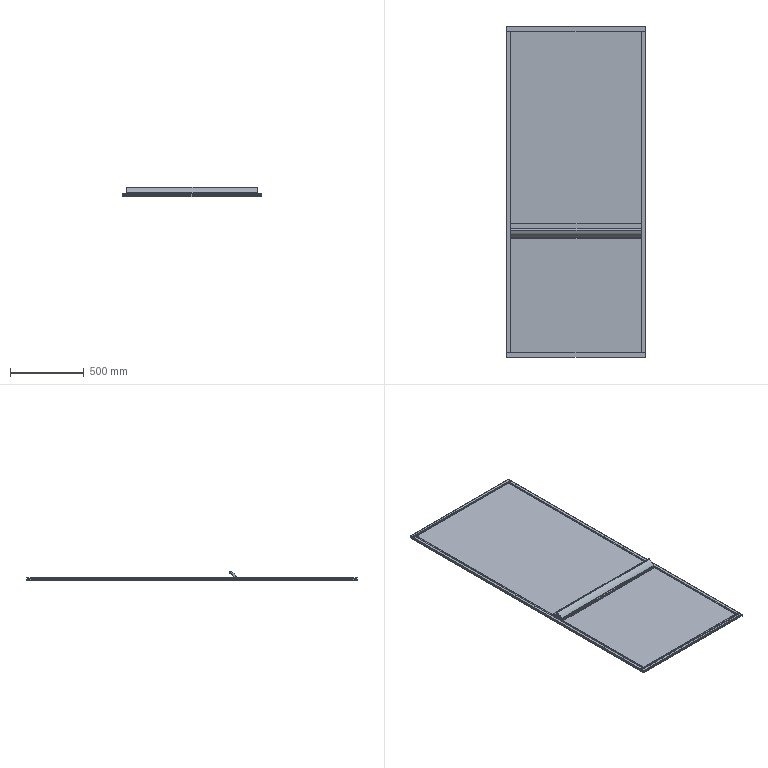Part | SolidWorks | features ICE 7, MirrorSolid 1, WeldMemberFeat 1, WeldmentFeature 1 | 13 solids | 408 faces | box 940 x 2236 x 62.186 mm | volume 20952715 mm3 | plane 252 | cylinder 156 | commonest cylinder face diameters 1.1 x36 3.6 x32 5.8 x29 4 x24 1 x10 0.4 x8